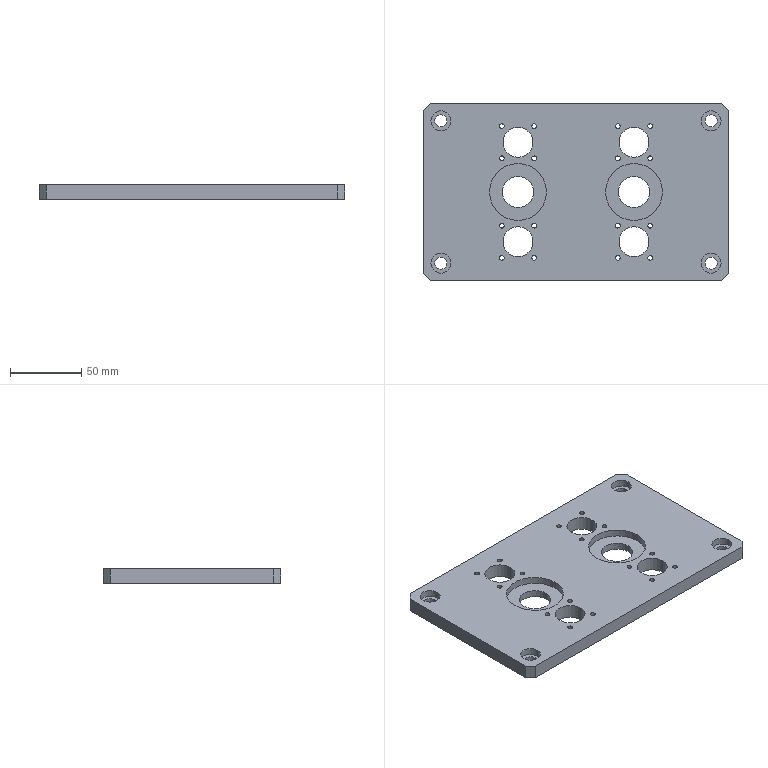CAM job | NX | 3-axis milling, drilling | part box 215 x 125 x 10 mm | stock box 215 x 125 x 10 mm
Tools:
number,name,description,diameter,corner_radius,flute_length,length,flutes
20,ZXZ,Milling Tool-5 Parameters,6.0,0.0,50.0,75.0,2
18,8.5ZT,Drilling Tool,8.5,0.0,35.0,50.0,2
13,3.3ZT,Drilling Tool,3.3,0.0,35.0,50.0,2
17,D17R0.8,Milling Tool-5 Parameters,17.0,0.8,50.0,75.0,2
3,D10,Milling Tool-5 Parameters,10.0,0.0,50.0,75.0,2
4,D10JING,Milling Tool-5 Parameters,10.0,0.0,50.0,75.0,2
2,D6A45,Milling Tool-5 Parameters,6.0,0.0,3.0,3.0,2
Operations:
program,operation,operation_type,tool,method,geometry_group,spindle_rpm,surface_speed,feed_per_tooth,feed_cut,feed_plunge,cut_length_mm,path_length_mm,cut_time_min,machine_time_min
1-215-125-10毛胚,DRILLING_COPY_1,Operation,ZXZ,METHOD,A,3000.0,56.0,0.0333,200.0,0.0,104.0,1048.421,0.52,0.6144
1-215-125-10毛胚,DRILLING_COPY_1_COPY_COPY_COPY_COPY,Operation,8.5ZT,METHOD,A,1200.0,33.0,0.0625,150.0,0.0,160.537,932.949,1.07,1.147
1-215-125-10毛胚,DRILLING_COPY_1_COPY_COPY_COPY_COPY_COPY_1,Operation,3.3ZT,METHOD,A,2000.0,20.0,0.025,100.0,0.0,247.863,1028.554,2.479,2.557
1-215-125-10毛胚,HOLE_MILLING,CylinderMilling,D17R0.8,METHOD,A,2000.0,106.0,0.5,2000.0,100.0,4743.987,5376.527,2.372,2.435
1-215-125-10毛胚,HOLE_MILLING_COPY,CylinderMilling,D17R0.8,METHOD,A,2000.0,106.0,0.5,2000.0,100.0,698.819,931.37,0.3494,0.3727
1-215-125-10毛胚,ZLEVEL_PROFILE_1_COPY_COPY_COPY_COPY,ZLevelMilling,D17R0.8,METHOD,A,2000.0,106.0,0.5,2000.0,2000.0,2329.27,3146.75,1.165,1.246
1-215-125-10毛胚,HOLE_MILLING_COPY_1,CylinderMilling,D10,METHOD,A,3000.0,94.0,0.3333,2000.0,100.0,1384.998,2057.707,0.6925,0.7598
1-215-125-10毛胚,ZLEVEL_PROFILE_COPY_COPY_1_COPY_COPY_COPY_1_COPY,ZLevelMilling,D10JING,METHOD,A,5000.0,157.0,0.1,1000.0,100.0,125.971,1289.499,0.126,0.2423
1-215-125-10毛胚,FLOOR_WALL_1_COPY_1,VolumeBased25DMillingOperation,D10JING,METHOD,A,5000.0,157.0,0.1,1000.0,100.0,484.905,698.498,0.4849,0.5063
1-215-125-10毛胚,ZLEVEL_PROFILE_COPY_1_COPY_COPY_COPY_COPY_2_COPY,ZLevelMilling,D6A45,METHOD,A,4000.0,75.0,0.125,1000.0,1000.0,1437.348,5430.409,1.437,1.837
1-215-125-10毛胚,ZLEVEL_PROFILE_COPY_1_COPY_COPY_COPY_COPY_2_COPY_COPY,ZLevelMilling,D6A45,METHOD,A,4000.0,75.0,0.125,1000.0,1000.0,233.419,1320.52,0.2334,0.3421
1-215-125-10毛胚,刀补4,ZLevelMilling,D10JING,METHOD,A,5000.0,157.0,0.08,800.0,100.0,160.477,708.692,0.2006,0.2554
1-215-125-10毛胚,刀补4_COPY,ZLevelMilling,D10JING,METHOD,A,5000.0,157.0,0.08,800.0,100.0,71.298,734.284,0.0891,0.1554